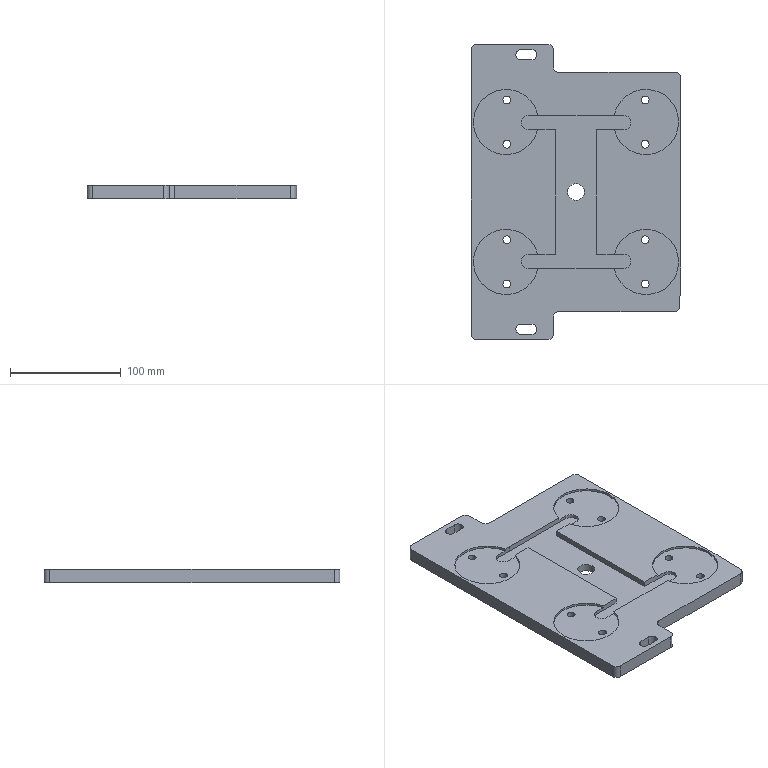Part | 1 solid | 73 faces | box 189.42 x 266.979 x 12 mm | volume 474902 mm3 | cylinder 44 | plane 29 | commonest cylinder face diameters 7 x16 10 x8 9 x6 13 x6 59 x6 15.25 x2